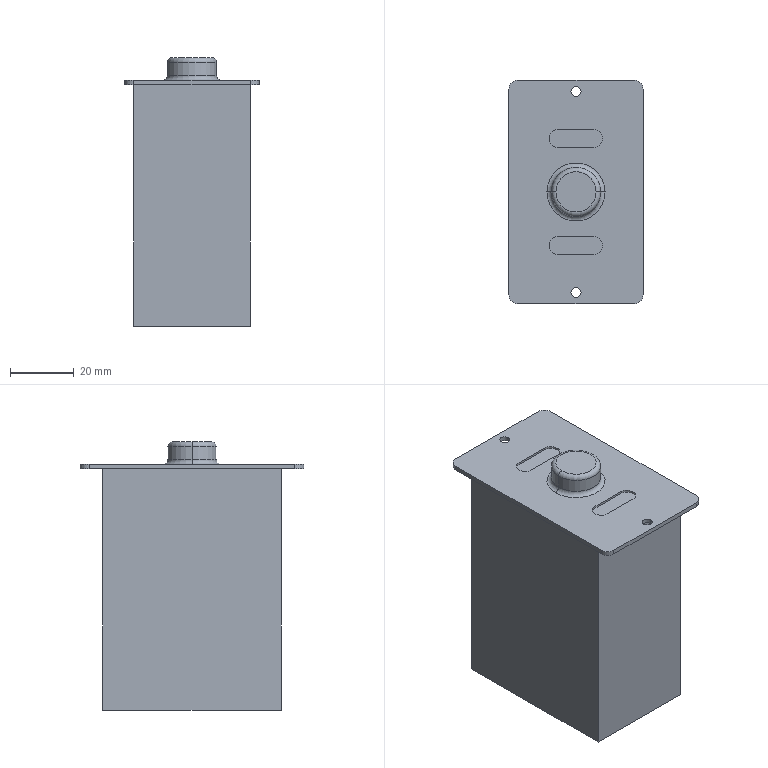Part | SolidWorks | features SplitBody 1 | 1 solid | 38 faces | box 42 x 70 x 84 mm | volume 159371 mm3 | plane 18 | cylinder 16 | torus 4 | commonest cylinder face diameters 5.6 x10 3.15 x4 15.4 x2
STEP:
#1=CARTESIAN_POINT('',(143.875,186.159,-254.516));
#2=VERTEX_POINT('',#1);
#3=CARTESIAN_POINT('',(125.675,186.159,-254.516));
#4=VERTEX_POINT('',#3);
#5=CARTESIAN_POINT('',(134.775,186.159,-254.516));
#6=DIRECTION('',(0.,0.,-1.));
#7=DIRECTION('',(-1.,0.,0.));
#8=AXIS2_PLACEMENT_3D('',#5,#6,#7);
#9=CIRCLE('',#8,9.1);
#10=EDGE_CURVE('',#2,#4,#9,.T.);
#11=ORIENTED_EDGE('',*,*,#10,.F.);
#12=CARTESIAN_POINT('',(142.475,186.159,-253.116));
#13=VERTEX_POINT('',#12);
#14=CARTESIAN_POINT('',(143.875,186.159,-253.116));
#15=DIRECTION('',(0.,1.,0.));
#16=DIRECTION('',(-1.,0.,0.));
#17=AXIS2_PLACEMENT_3D('',#14,#15,#16);
#18=CIRCLE('',#17,1.4);
#19=EDGE_CURVE('',#2,#13,#18,.T.);
#20=ORIENTED_EDGE('',*,*,#19,.T.);
#21=CARTESIAN_POINT('',(127.075,186.159,-253.116));
#22=VERTEX_POINT('',#21);
#23=CARTESIAN_POINT('',(134.775,186.159,-253.116));
#24=DIRECTION('',(0.,0.,1.));
#25=DIRECTION('',(-1.,0.,0.));
#26=AXIS2_PLACEMENT_3D('',#23,#24,#25);
#27=CIRCLE('',#26,7.7);
#28=EDGE_CURVE('',#22,#13,#27,.T.);
#29=ORIENTED_EDGE('',*,*,#28,.F.);
#30=CARTESIAN_POINT('',(125.675,186.159,-253.116));
#31=DIRECTION('',(0.,-1.,0.));
#32=DIRECTION('',(1.,0.,0.));
#33=AXIS2_PLACEMENT_3D('',#30,#31,#32);
#34=CIRCLE('',#33,1.4);
#35=EDGE_CURVE('',#4,#22,#34,.T.);
#36=ORIENTED_EDGE('',*,*,#35,.F.);
#37=EDGE_LOOP('',(#11,#20,#29,#36));
#38=FACE_OUTER_BOUND('',#37,.T.);
#39=CARTESIAN_POINT('',(134.775,186.159,-253.116));
#40=DIRECTION('',(0.,0.,-1.));
#41=DIRECTION('',(-1.,0.,0.));
#42=AXIS2_PLACEMENT_3D('',#39,#40,#41);
#43=TOROIDAL_SURFACE('',#42,9.1,1.4);
#44=ADVANCED_FACE('',(#38),#43,.F.);
#45=CARTESIAN_POINT('',(127.075,186.159,-248.916));
#46=VERTEX_POINT('',#45);
#47=CARTESIAN_POINT('',(142.475,186.159,-248.916));
#48=VERTEX_POINT('',#47);
#49=CARTESIAN_POINT('',(134.775,186.159,-248.916));
#50=DIRECTION('',(0.,0.,-1.));
#51=DIRECTION('',(1.,0.,0.));
#52=AXIS2_PLACEMENT_3D('',#49,#50,#51);
#53=CIRCLE('',#52,7.7);
#54=EDGE_CURVE('',#46,#48,#53,.T.);
#55=ORIENTED_EDGE('',*,*,#54,.F.);
#56=CARTESIAN_POINT('',(128.475,186.159,-247.516));
#57=VERTEX_POINT('',#56);
#58=CARTESIAN_POINT('',(128.475,186.159,-248.916));
#59=DIRECTION('',(0.,1.,0.));
#60=DIRECTION('',(0.,0.,1.));
#61=AXIS2_PLACEMENT_3D('',#58,#59,#60);
#62=CIRCLE('',#61,1.4);
#63=EDGE_CURVE('',#46,#57,#62,.T.);
#64=ORIENTED_EDGE('',*,*,#63,.T.);
#65=CARTESIAN_POINT('',(141.075,186.159,-247.516));
#66=VERTEX_POINT('',#65);
#67=CARTESIAN_POINT('',(134.775,186.159,-247.516));
#68=DIRECTION('',(0.,0.,1.));
#69=DIRECTION('',(1.,0.,0.));
#70=AXIS2_PLACEMENT_3D('',#67,#68,#69);
#71=CIRCLE('',#70,6.3);
#72=EDGE_CURVE('',#66,#57,#71,.T.);
#73=ORIENTED_EDGE('',*,*,#72,.F.);
#74=CARTESIAN_POINT('',(141.075,186.159,-248.916));
#75=DIRECTION('',(0.,-1.,0.));
#76=DIRECTION('',(1.,0.,0.));
#77=AXIS2_PLACEMENT_3D('',#74,#75,#76);
#78=CIRCLE('',#77,1.4);
#79=EDGE_CURVE('',#48,#66,#78,.T.);
#80=ORIENTED_EDGE('',*,*,#79,.F.);
#81=EDGE_LOOP('',(#55,#64,#73,#80));
#82=FACE_OUTER_BOUND('',#81,.T.);
#83=CARTESIAN_POINT('',(134.775,186.159,-248.916));
#84=DIRECTION('',(0.,0.,1.));
#85=DIRECTION('',(1.,0.,0.));
#86=AXIS2_PLACEMENT_3D('',#83,#84,#85);
#87=TOROIDAL_SURFACE('',#86,6.3,1.4);
#88=ADVANCED_FACE('',(#82),#87,.T.);
#89=CARTESIAN_POINT('',(143.175,169.359,-255.216));
#90=VERTEX_POINT('',#89);
#91=CARTESIAN_POINT('',(140.375,172.159,-255.216));
#92=VERTEX_POINT('',#91);
#93=CARTESIAN_POINT('',(140.375,169.359,-255.216));
#94=DIRECTION('',(0.,0.,1.));
#95=DIRECTION('',(-1.,0.,0.));
#96=AXIS2_PLACEMENT_3D('',#93,#94,#95);
#97=CIRCLE('',#96,2.8);
#98=EDGE_CURVE('',#90,#92,#97,.T.);
#99=ORIENTED_EDGE('',*,*,#98,.F.);
#100=CARTESIAN_POINT('',(143.175,169.359,-254.516));
#101=VERTEX_POINT('',#100);
#102=CARTESIAN_POINT('',(143.175,169.359,-255.216));
#103=DIRECTION('',(0.,0.,1.));
#104=VECTOR('',#103,1000.);
#105=LINE('',#102,#104);
#106=EDGE_CURVE('',#90,#101,#105,.T.);
#107=ORIENTED_EDGE('',*,*,#106,.T.);
#108=CARTESIAN_POINT('',(140.375,172.159,-254.516));
#109=VERTEX_POINT('',#108);
#110=CARTESIAN_POINT('',(140.375,169.359,-254.516));
#111=DIRECTION('',(0.,0.,1.));
#112=DIRECTION('',(-1.,0.,0.));
#113=AXIS2_PLACEMENT_3D('',#110,#111,#112);
#114=CIRCLE('',#113,2.8);
#115=EDGE_CURVE('',#101,#109,#114,.T.);
#116=ORIENTED_EDGE('',*,*,#115,.T.);
#117=CARTESIAN_POINT('',(140.375,172.159,-255.216));
#118=DIRECTION('',(0.,0.,1.));
#119=VECTOR('',#118,1000.);
#120=LINE('',#117,#119);
#121=EDGE_CURVE('',#92,#109,#120,.T.);
#122=ORIENTED_EDGE('',*,*,#121,.F.);
#123=EDGE_LOOP('',(#99,#107,#116,#122));
#124=FACE_OUTER_BOUND('',#123,.T.);
#125=CARTESIAN_POINT('',(140.375,169.359,-255.216));
#126=DIRECTION('',(0.,0.,1.));
#127=DIRECTION('',(1.,0.,0.));
#128=AXIS2_PLACEMENT_3D('',#125,#126,#127);
#129=CYLINDRICAL_SURFACE('',#128,2.8);
#130=ADVANCED_FACE('',(#124),#129,.F.);
#131=CARTESIAN_POINT('',(143.175,202.959,-255.216));
#132=VERTEX_POINT('',#131);
#133=CARTESIAN_POINT('',(140.375,205.759,-255.216));
#134=VERTEX_POINT('',#133);
#135=CARTESIAN_POINT('',(140.375,202.959,-255.216));
#136=DIRECTION('',(0.,0.,1.));
#137=DIRECTION('',(1.,0.,0.));
#138=AXIS2_PLACEMENT_3D('',#135,#136,#137);
#139=CIRCLE('',#138,2.8);
#140=EDGE_CURVE('',#132,#134,#139,.T.);
#141=ORIENTED_EDGE('',*,*,#140,.F.);
#142=CARTESIAN_POINT('',(143.175,202.959,-254.516));
#143=VERTEX_POINT('',#142);
#144=CARTESIAN_POINT('',(143.175,202.959,-255.216));
#145=DIRECTION('',(0.,0.,1.));
#146=VECTOR('',#145,1000.);
#147=LINE('',#144,#146);
#148=EDGE_CURVE('',#132,#143,#147,.T.);
#149=ORIENTED_EDGE('',*,*,#148,.T.);
#150=CARTESIAN_POINT('',(140.375,205.759,-254.516));
#151=VERTEX_POINT('',#150);
#152=CARTESIAN_POINT('',(140.375,202.959,-254.516));
#153=DIRECTION('',(0.,0.,1.));
#154=DIRECTION('',(1.,0.,0.));
#155=AXIS2_PLACEMENT_3D('',#152,#153,#154);
#156=CIRCLE('',#155,2.8);
#157=EDGE_CURVE('',#143,#151,#156,.T.);
#158=ORIENTED_EDGE('',*,*,#157,.T.);
#159=CARTESIAN_POINT('',(140.375,205.759,-255.216));
#160=DIRECTION('',(0.,0.,1.));
#161=VECTOR('',#160,1000.);
#162=LINE('',#159,#161);
#163=EDGE_CURVE('',#134,#151,#162,.T.);
#164=ORIENTED_EDGE('',*,*,#163,.F.);
#165=EDGE_LOOP('',(#141,#149,#158,#164));
#166=FACE_OUTER_BOUND('',#165,.T.);
#167=CARTESIAN_POINT('',(140.375,202.959,-255.216));
#168=DIRECTION('',(0.,0.,1.));
#169=DIRECTION('',(1.,0.,0.));
#170=AXIS2_PLACEMENT_3D('',#167,#168,#169);
#171=CYLINDRICAL_SURFACE('',#170,2.8);
#172=ADVANCED_FACE('',(#166),#171,.F.);
#173=ORIENTED_EDGE('',*,*,#54,.T.);
#174=CARTESIAN_POINT('',(142.475,186.159,-247.516));
#175=DIRECTION('',(0.,0.,-1.));
#176=VECTOR('',#175,1000.);
#177=LINE('',#174,#176);
#178=EDGE_CURVE('',#48,#13,#177,.T.);
#179=ORIENTED_EDGE('',*,*,#178,.T.);
#180=CARTESIAN_POINT('',(134.775,186.159,-253.116));
#181=DIRECTION('',(0.,0.,1.));
#182=DIRECTION('',(-1.,0.,0.));
#183=AXIS2_PLACEMENT_3D('',#180,#181,#182);
#184=CIRCLE('',#183,7.7);
#185=EDGE_CURVE('',#13,#22,#184,.T.);
#186=ORIENTED_EDGE('',*,*,#185,.T.);
#187=CARTESIAN_POINT('',(127.075,186.159,-247.516));
#188=DIRECTION('',(0.,0.,-1.));
#189=VECTOR('',#188,1000.);
#190=LINE('',#187,#189);
#191=EDGE_CURVE('',#46,#22,#190,.T.);
#192=ORIENTED_EDGE('',*,*,#191,.F.);
#193=EDGE_LOOP('',(#173,#179,#186,#192));
#194=FACE_OUTER_BOUND('',#193,.T.);
#195=CARTESIAN_POINT('',(134.775,186.159,-247.516));
#196=DIRECTION('',(0.,0.,-1.));
#197=DIRECTION('',(-1.,0.,0.));
#198=AXIS2_PLACEMENT_3D('',#195,#196,#197);
#199=CYLINDRICAL_SURFACE('',#198,7.7);
#200=ADVANCED_FACE('',(#194),#199,.T.);
#201=CARTESIAN_POINT('',(133.2,154.659,-255.916));
#202=VERTEX_POINT('',#201);
#203=CARTESIAN_POINT('',(136.35,154.659,-255.916));
#204=VERTEX_POINT('',#203);
#205=CARTESIAN_POINT('',(134.775,154.659,-255.916));
#206=DIRECTION('',(0.,0.,1.));
#207=DIRECTION('',(1.,0.,0.));
#208=AXIS2_PLACEMENT_3D('',#205,#206,#207);
#209=CIRCLE('',#208,1.575);
#210=EDGE_CURVE('',#202,#204,#209,.T.);
#211=ORIENTED_EDGE('',*,*,#210,.F.);
#212=CARTESIAN_POINT('',(133.2,154.659,-254.516));
#213=VERTEX_POINT('',#212);
#214=CARTESIAN_POINT('',(133.2,154.659,-331.516));
#215=DIRECTION('',(0.,0.,1.));
#216=VECTOR('',#215,1000.);
#217=LINE('',#214,#216);
#218=EDGE_CURVE('',#202,#213,#217,.T.);
#219=ORIENTED_EDGE('',*,*,#218,.T.);
#220=CARTESIAN_POINT('',(136.35,154.659,-254.516));
#221=VERTEX_POINT('',#220);
#222=CARTESIAN_POINT('',(134.775,154.659,-254.516));
#223=DIRECTION('',(0.,0.,1.));
#224=DIRECTION('',(-1.,0.,0.));
#225=AXIS2_PLACEMENT_3D('',#222,#223,#224);
#226=CIRCLE('',#225,1.575);
#227=EDGE_CURVE('',#213,#221,#226,.T.);
#228=ORIENTED_EDGE('',*,*,#227,.T.);
#229=CARTESIAN_POINT('',(136.35,154.659,-331.516));
#230=DIRECTION('',(0.,0.,1.));
#231=VECTOR('',#230,1000.);
#232=LINE('',#229,#231);
#233=EDGE_CURVE('',#204,#221,#232,.T.);
#234=ORIENTED_EDGE('',*,*,#233,.F.);
#235=EDGE_LOOP('',(#211,#219,#228,#234));
#236=FACE_OUTER_BOUND('',#235,.T.);
#237=CARTESIAN_POINT('',(134.775,154.659,-331.516));
#238=DIRECTION('',(0.,0.,1.));
#239=DIRECTION('',(1.,0.,0.));
#240=AXIS2_PLACEMENT_3D('',#237,#238,#239);
#241=CYLINDRICAL_SURFACE('',#240,1.575);
#242=ADVANCED_FACE('',(#236),#241,.F.);
#243=CARTESIAN_POINT('',(133.2,217.659,-255.916));
#244=VERTEX_POINT('',#243);
#245=CARTESIAN_POINT('',(136.35,217.659,-255.916));
#246=VERTEX_POINT('',#245);
#247=CARTESIAN_POINT('',(134.775,217.659,-255.916));
#248=DIRECTION('',(0.,0.,1.));
#249=DIRECTION('',(1.,0.,0.));
#250=AXIS2_PLACEMENT_3D('',#247,#248,#249);
#251=CIRCLE('',#250,1.575);
#252=EDGE_CURVE('',#244,#246,#251,.T.);
#253=ORIENTED_EDGE('',*,*,#252,.F.);
#254=CARTESIAN_POINT('',(133.2,217.659,-254.516));
#255=VERTEX_POINT('',#254);
#256=CARTESIAN_POINT('',(133.2,217.659,-331.516));
#257=DIRECTION('',(0.,0.,1.));
#258=VECTOR('',#257,1000.);
#259=LINE('',#256,#258);
#260=EDGE_CURVE('',#244,#255,#259,.T.);
#261=ORIENTED_EDGE('',*,*,#260,.T.);
#262=CARTESIAN_POINT('',(136.35,217.659,-254.516));
#263=VERTEX_POINT('',#262);
#264=CARTESIAN_POINT('',(134.775,217.659,-254.516));
#265=DIRECTION('',(0.,0.,1.));
#266=DIRECTION('',(1.,0.,0.));
#267=AXIS2_PLACEMENT_3D('',#264,#265,#266);
#268=CIRCLE('',#267,1.575);
#269=EDGE_CURVE('',#255,#263,#268,.T.);
#270=ORIENTED_EDGE('',*,*,#269,.T.);
#271=CARTESIAN_POINT('',(136.35,217.659,-331.516));
#272=DIRECTION('',(0.,0.,1.));
#273=VECTOR('',#272,1000.);
#274=LINE('',#271,#273);
#275=EDGE_CURVE('',#246,#263,#274,.T.);
#276=ORIENTED_EDGE('',*,*,#275,.F.);
#277=EDGE_LOOP('',(#253,#261,#270,#276));
#278=FACE_OUTER_BOUND('',#277,.T.);
#279=CARTESIAN_POINT('',(134.775,217.659,-331.516));
#280=DIRECTION('',(0.,0.,1.));
#281=DIRECTION('',(1.,0.,0.));
#282=AXIS2_PLACEMENT_3D('',#279,#280,#281);
#283=CYLINDRICAL_SURFACE('',#282,1.575);
#284=ADVANCED_FACE('',(#278),#283,.F.);
#285=CARTESIAN_POINT('',(134.775,186.159,-254.516));
#286=DIRECTION('',(0.,0.,-1.));
#287=DIRECTION('',(-1.,0.,0.));
#288=AXIS2_PLACEMENT_3D('',#285,#286,#287);
#289=CIRCLE('',#288,9.1);
#290=EDGE_CURVE('',#4,#2,#289,.T.);
#291=ORIENTED_EDGE('',*,*,#290,.T.);
#292=ORIENTED_EDGE('',*,*,#10,.T.);
#293=EDGE_LOOP('',(#291,#292));
#294=FACE_BOUND('',#293,.T.);
#295=CARTESIAN_POINT('',(129.175,166.559,-254.516));
#296=VERTEX_POINT('',#295);
#297=CARTESIAN_POINT('',(140.375,166.559,-254.516));
#298=VERTEX_POINT('',#297);
#299=CARTESIAN_POINT('',(129.175,166.559,-254.516));
#300=DIRECTION('',(1.,0.,0.));
#301=VECTOR('',#300,1000.);
#302=LINE('',#299,#301);
#303=EDGE_CURVE('',#296,#298,#302,.T.);
#304=ORIENTED_EDGE('',*,*,#303,.F.);
#305=CARTESIAN_POINT('',(129.175,172.159,-254.516));
#306=VERTEX_POINT('',#305);
#307=CARTESIAN_POINT('',(129.175,169.359,-254.516));
#308=DIRECTION('',(0.,0.,1.));
#309=DIRECTION('',(-1.,0.,0.));
#310=AXIS2_PLACEMENT_3D('',#307,#308,#309);
#311=CIRCLE('',#310,2.8);
#312=EDGE_CURVE('',#306,#296,#311,.T.);
#313=ORIENTED_EDGE('',*,*,#312,.F.);
#314=CARTESIAN_POINT('',(129.175,172.159,-254.516));
#315=DIRECTION('',(-1.,0.,0.));
#316=VECTOR('',#315,1000.);
#317=LINE('',#314,#316);
#318=EDGE_CURVE('',#109,#306,#317,.T.);
#319=ORIENTED_EDGE('',*,*,#318,.F.);
#320=ORIENTED_EDGE('',*,*,#115,.F.);
#321=CARTESIAN_POINT('',(140.375,169.359,-254.516));
#322=DIRECTION('',(0.,0.,1.));
#323=DIRECTION('',(-1.,0.,0.));
#324=AXIS2_PLACEMENT_3D('',#321,#322,#323);
#325=CIRCLE('',#324,2.8);
#326=EDGE_CURVE('',#298,#101,#325,.T.);
#327=ORIENTED_EDGE('',*,*,#326,.F.);
#328=EDGE_LOOP('',(#304,#313,#319,#320,#327));
#329=FACE_BOUND('',#328,.T.);
#330=CARTESIAN_POINT('',(129.175,200.159,-254.516));
#331=VERTEX_POINT('',#330);
#332=CARTESIAN_POINT('',(140.375,200.159,-254.516));
#333=VERTEX_POINT('',#332);
#334=CARTESIAN_POINT('',(129.175,200.159,-254.516));
#335=DIRECTION('',(1.,0.,0.));
#336=VECTOR('',#335,1000.);
#337=LINE('',#334,#336);
#338=EDGE_CURVE('',#331,#333,#337,.T.);
#339=ORIENTED_EDGE('',*,*,#338,.F.);
#340=CARTESIAN_POINT('',(129.175,205.759,-254.516));
#341=VERTEX_POINT('',#340);
#342=CARTESIAN_POINT('',(129.175,202.959,-254.516));
#343=DIRECTION('',(0.,0.,1.));
#344=DIRECTION('',(1.,0.,0.));
#345=AXIS2_PLACEMENT_3D('',#342,#343,#344);
#346=CIRCLE('',#345,2.8);
#347=EDGE_CURVE('',#341,#331,#346,.T.);
#348=ORIENTED_EDGE('',*,*,#347,.F.);
#349=CARTESIAN_POINT('',(129.175,205.759,-254.516));
#350=DIRECTION('',(-1.,0.,0.));
#351=VECTOR('',#350,1000.);
#352=LINE('',#349,#351);
#353=EDGE_CURVE('',#151,#341,#352,.T.);
#354=ORIENTED_EDGE('',*,*,#353,.F.);
#355=ORIENTED_EDGE('',*,*,#157,.F.);
#356=CARTESIAN_POINT('',(140.375,202.959,-254.516));
#357=DIRECTION('',(0.,0.,1.));
#358=DIRECTION('',(1.,0.,0.));
#359=AXIS2_PLACEMENT_3D('',#356,#357,#358);
#360=CIRCLE('',#359,2.8);
#361=EDGE_CURVE('',#333,#143,#360,.T.);
#362=ORIENTED_EDGE('',*,*,#361,.F.);
#363=EDGE_LOOP('',(#339,#348,#354,#355,#362));
#364=FACE_BOUND('',#363,.T.);
#365=CARTESIAN_POINT('',(116.575,151.159,-254.516));
#366=VERTEX_POINT('',#365);
#367=CARTESIAN_POINT('',(152.975,151.159,-254.516));
#368=VERTEX_POINT('',#367);
#369=CARTESIAN_POINT('',(113.775,151.159,-254.516));
#370=DIRECTION('',(1.,0.,0.));
#371=VECTOR('',#370,1000.);
#372=LINE('',#369,#371);
#373=EDGE_CURVE('',#366,#368,#372,.T.);
#374=ORIENTED_EDGE('',*,*,#373,.T.);
#375=CARTESIAN_POINT('',(155.775,153.959,-254.516));
#376=VERTEX_POINT('',#375);
#377=CARTESIAN_POINT('',(152.975,153.959,-254.516));
#378=DIRECTION('',(0.,0.,1.));
#379=DIRECTION('',(-1.,0.,0.));
#380=AXIS2_PLACEMENT_3D('',#377,#378,#379);
#381=CIRCLE('',#380,2.8);
#382=EDGE_CURVE('',#368,#376,#381,.T.);
#383=ORIENTED_EDGE('',*,*,#382,.T.);
#384=CARTESIAN_POINT('',(155.775,218.359,-254.516));
#385=VERTEX_POINT('',#384);
#386=CARTESIAN_POINT('',(155.775,221.159,-254.516));
#387=DIRECTION('',(0.,1.,0.));
#388=VECTOR('',#387,1000.);
#389=LINE('',#386,#388);
#390=EDGE_CURVE('',#376,#385,#389,.T.);
#391=ORIENTED_EDGE('',*,*,#390,.T.);
#392=CARTESIAN_POINT('',(152.975,221.159,-254.516));
#393=VERTEX_POINT('',#392);
#394=CARTESIAN_POINT('',(152.975,218.359,-254.516));
#395=DIRECTION('',(0.,0.,1.));
#396=DIRECTION('',(-1.,0.,0.));
#397=AXIS2_PLACEMENT_3D('',#394,#395,#396);
#398=CIRCLE('',#397,2.8);
#399=EDGE_CURVE('',#385,#393,#398,.T.);
#400=ORIENTED_EDGE('',*,*,#399,.T.);
#401=CARTESIAN_POINT('',(116.575,221.159,-254.516));
#402=VERTEX_POINT('',#401);
#403=CARTESIAN_POINT('',(113.775,221.159,-254.516));
#404=DIRECTION('',(-1.,0.,0.));
#405=VECTOR('',#404,1000.);
#406=LINE('',#403,#405);
#407=EDGE_CURVE('',#393,#402,#406,.T.);
#408=ORIENTED_EDGE('',*,*,#407,.T.);
#409=CARTESIAN_POINT('',(113.775,218.359,-254.516));
#410=VERTEX_POINT('',#409);
#411=CARTESIAN_POINT('',(116.575,218.359,-254.516));
#412=DIRECTION('',(0.,0.,1.));
#413=DIRECTION('',(-1.,0.,0.));
#414=AXIS2_PLACEMENT_3D('',#411,#412,#413);
#415=CIRCLE('',#414,2.8);
#416=EDGE_CURVE('',#402,#410,#415,.T.);
#417=ORIENTED_EDGE('',*,*,#416,.T.);
#418=CARTESIAN_POINT('',(113.775,153.959,-254.516));
#419=VERTEX_POINT('',#418);
#420=CARTESIAN_POINT('',(113.775,221.159,-254.516));
#421=DIRECTION('',(0.,-1.,0.));
#422=VECTOR('',#421,1000.);
#423=LINE('',#420,#422);
#424=EDGE_CURVE('',#410,#419,#423,.T.);
#425=ORIENTED_EDGE('',*,*,#424,.T.);
#426=CARTESIAN_POINT('',(116.575,153.959,-254.516));
#427=DIRECTION('',(0.,0.,1.));
#428=DIRECTION('',(-1.,0.,0.));
#429=AXIS2_PLACEMENT_3D('',#426,#427,#428);
#430=CIRCLE('',#429,2.8);
#431=EDGE_CURVE('',#419,#366,#430,.T.);
#432=ORIENTED_EDGE('',*,*,#431,.T.);
#433=EDGE_LOOP('',(#374,#383,#391,#400,#408,#417,#425,#432));
#434=FACE_OUTER_BOUND('',#433,.T.);
#435=CARTESIAN_POINT('',(134.775,217.659,-254.516));
#436=DIRECTION('',(0.,0.,1.));
#437=DIRECTION('',(1.,0.,0.));
#438=AXIS2_PLACEMENT_3D('',#435,#436,#437);
#439=CIRCLE('',#438,1.575);
#440=EDGE_CURVE('',#263,#255,#439,.T.);
#441=ORIENTED_EDGE('',*,*,#440,.F.);
#442=ORIENTED_EDGE('',*,*,#269,.F.);
#443=EDGE_LOOP('',(#441,#442));
#444=FACE_BOUND('',#443,.T.);
#445=CARTESIAN_POINT('',(134.775,154.659,-254.516));
#446=DIRECTION('',(0.,0.,1.));
#447=DIRECTION('',(-1.,0.,0.));
#448=AXIS2_PLACEMENT_3D('',#445,#446,#447);
#449=CIRCLE('',#448,1.575);
#450=EDGE_CURVE('',#221,#213,#449,.T.);
#451=ORIENTED_EDGE('',*,*,#450,.F.);
#452=ORIENTED_EDGE('',*,*,#227,.F.);
#453=EDGE_LOOP('',(#451,#452));
#454=FACE_BOUND('',#453,.T.);
#455=CARTESIAN_POINT('',(152.975,158.159,-254.516));
#456=DIRECTION('',(0.,0.,-1.));
#457=DIRECTION('',(-1.,0.,0.));
#458=AXIS2_PLACEMENT_3D('',#455,#456,#457);
#459=PLANE('',#458);
#460=ADVANCED_FACE('',(#294,#329,#364,#434,#444,#454),#459,.F.);
#461=CARTESIAN_POINT('',(152.975,158.159,-255.916));
#462=VERTEX_POINT('',#461);
#463=CARTESIAN_POINT('',(152.975,214.159,-255.916));
#464=VERTEX_POINT('',#463);
#465=CARTESIAN_POINT('',(152.975,214.159,-255.916));
#466=DIRECTION('',(0.,1.,0.));
#467=VECTOR('',#466,1000.);
#468=LINE('',#465,#467);
#469=EDGE_CURVE('',#462,#464,#468,.T.);
#470=ORIENTED_EDGE('',*,*,#469,.F.);
#471=CARTESIAN_POINT('',(152.975,158.159,-331.516));
#472=VERTEX_POINT('',#471);
#473=CARTESIAN_POINT('',(152.975,158.159,-331.516));
#474=DIRECTION('',(0.,0.,1.));
#475=VECTOR('',#474,1000.);
#476=LINE('',#473,#475);
#477=EDGE_CURVE('',#472,#462,#476,.T.);
#478=ORIENTED_EDGE('',*,*,#477,.F.);
#479=CARTESIAN_POINT('',(152.975,214.159,-331.516));
#480=VERTEX_POINT('',#479);
#481=CARTESIAN_POINT('',(152.975,214.159,-331.516));
#482=DIRECTION('',(0.,-1.,0.));
#483=VECTOR('',#482,1000.);
#484=LINE('',#481,#483);
#485=EDGE_CURVE('',#480,#472,#484,.T.);
#486=ORIENTED_EDGE('',*,*,#485,.F.);
#487=CARTESIAN_POINT('',(152.975,214.159,-331.516));
#488=DIRECTION('',(0.,0.,1.));
#489=VECTOR('',#488,1000.);
#490=LINE('',#487,#489);
#491=EDGE_CURVE('',#480,#464,#490,.T.);
#492=ORIENTED_EDGE('',*,*,#491,.T.);
#493=EDGE_LOOP('',(#470,#478,#486,#492));
#494=FACE_OUTER_BOUND('',#493,.T.);
#495=CARTESIAN_POINT('',(152.975,214.159,-331.516));
#496=DIRECTION('',(-1.,0.,0.));
#497=DIRECTION('',(0.,1.,0.));
#498=AXIS2_PLACEMENT_3D('',#495,#496,#497);
#499=PLANE('',#498);
#500=ADVANCED_FACE('',(#494),#499,.F.);
#501=CARTESIAN_POINT('',(116.575,158.159,-255.916));
#502=VERTEX_POINT('',#501);
#503=CARTESIAN_POINT('',(152.975,158.159,-255.916));
#504=DIRECTION('',(1.,0.,0.));
#505=VECTOR('',#504,1000.);
#506=LINE('',#503,#505);
#507=EDGE_CURVE('',#502,#462,#506,.T.);
#508=ORIENTED_EDGE('',*,*,#507,.F.);
#509=CARTESIAN_POINT('',(116.575,158.159,-331.516));
#510=VERTEX_POINT('',#509);
#511=CARTESIAN_POINT('',(116.575,158.159,-331.516));
#512=DIRECTION('',(0.,0.,1.));
#513=VECTOR('',#512,1000.);
#514=LINE('',#511,#513);
#515=EDGE_CURVE('',#510,#502,#514,.T.);
#516=ORIENTED_EDGE('',*,*,#515,.F.);
#517=CARTESIAN_POINT('',(152.975,158.159,-331.516));
#518=DIRECTION('',(-1.,0.,0.));
#519=VECTOR('',#518,1000.);
#520=LINE('',#517,#519);
#521=EDGE_CURVE('',#472,#510,#520,.T.);
#522=ORIENTED_EDGE('',*,*,#521,.F.);
#523=ORIENTED_EDGE('',*,*,#477,.T.);
#524=EDGE_LOOP('',(#508,#516,#522,#523));
#525=FACE_OUTER_BOUND('',#524,.T.);
#526=CARTESIAN_POINT('',(152.975,158.159,-331.516));
#527=DIRECTION('',(0.,1.,0.));
#528=DIRECTION('',(0.,0.,-1.));
#529=AXIS2_PLACEMENT_3D('',#526,#527,#528);
#530=PLANE('',#529);
#531=ADVANCED_FACE('',(#525),#530,.F.);
#532=CARTESIAN_POINT('',(116.575,214.159,-255.916));
#533=VERTEX_POINT('',#532);
#534=CARTESIAN_POINT('',(116.575,214.159,-255.916));
#535=DIRECTION('',(0.,-1.,0.));
#536=VECTOR('',#535,1000.);
#537=LINE('',#534,#536);
#538=EDGE_CURVE('',#533,#502,#537,.T.);
#539=ORIENTED_EDGE('',*,*,#538,.F.);
#540=CARTESIAN_POINT('',(116.575,214.159,-331.516));
#541=VERTEX_POINT('',#540);
#542=CARTESIAN_POINT('',(116.575,214.159,-331.516));
#543=DIRECTION('',(0.,0.,1.));
#544=VECTOR('',#543,1000.);
#545=LINE('',#542,#544);
#546=EDGE_CURVE('',#541,#533,#545,.T.);
#547=ORIENTED_EDGE('',*,*,#546,.F.);
#548=CARTESIAN_POINT('',(116.575,214.159,-331.516));
#549=DIRECTION('',(0.,1.,0.));
#550=VECTOR('',#549,1000.);
#551=LINE('',#548,#550);
#552=EDGE_CURVE('',#510,#541,#551,.T.);
#553=ORIENTED_EDGE('',*,*,#552,.F.);
#554=ORIENTED_EDGE('',*,*,#515,.T.);
#555=EDGE_LOOP('',(#539,#547,#553,#554));
#556=FACE_OUTER_BOUND('',#555,.T.);
#557=CARTESIAN_POINT('',(116.575,214.159,-331.516));
#558=DIRECTION('',(1.,0.,0.));
#559=DIRECTION('',(0.,-1.,0.));
#560=AXIS2_PLACEMENT_3D('',#557,#558,#559);
#561=PLANE('',#560);
#562=ADVANCED_FACE('',(#556),#561,.F.);
#563=CARTESIAN_POINT('',(152.975,214.159,-255.916));
#564=DIRECTION('',(-1.,0.,0.));
#565=VECTOR('',#564,1000.);
#566=LINE('',#563,#565);
#567=EDGE_CURVE('',#464,#533,#566,.T.);
#568=ORIENTED_EDGE('',*,*,#567,.F.);
#569=ORIENTED_EDGE('',*,*,#491,.F.);
#570=CARTESIAN_POINT('',(152.975,214.159,-331.516));
#571=DIRECTION('',(1.,0.,0.));
#572=VECTOR('',#571,1000.);
#573=LINE('',#570,#572);
#574=EDGE_CURVE('',#541,#480,#573,.T.);
#575=ORIENTED_EDGE('',*,*,#574,.F.);
#576=ORIENTED_EDGE('',*,*,#546,.T.);
#577=EDGE_LOOP('',(#568,#569,#575,#576));
#578=FACE_OUTER_BOUND('',#577,.T.);
#579=CARTESIAN_POINT('',(152.975,214.159,-331.516));
#580=DIRECTION('',(0.,-1.,0.));
#581=DIRECTION('',(0.,0.,1.));
#582=AXIS2_PLACEMENT_3D('',#579,#580,#581);
#583=PLANE('',#582);
#584=ADVANCED_FACE('',(#578),#583,.F.);
#585=ORIENTED_EDGE('',*,*,#485,.T.);
#586=ORIENTED_EDGE('',*,*,#521,.T.);
#587=ORIENTED_EDGE('',*,*,#552,.T.);
#588=ORIENTED_EDGE('',*,*,#574,.T.);
#589=EDGE_LOOP('',(#585,#586,#587,#588));
#590=FACE_OUTER_BOUND('',#589,.T.);
#591=CARTESIAN_POINT('',(152.975,158.159,-331.516));
#592=DIRECTION('',(0.,0.,-1.));
#593=DIRECTION('',(-1.,0.,0.));
#594=AXIS2_PLACEMENT_3D('',#591,#592,#593);
#595=PLANE('',#594);
#596=ADVANCED_FACE('',(#590),#595,.T.);
#597=CARTESIAN_POINT('',(134.775,154.659,-255.916));
#598=DIRECTION('',(0.,0.,1.));
#599=DIRECTION('',(1.,0.,0.));
#600=AXIS2_PLACEMENT_3D('',#597,#598,#599);
#601=CIRCLE('',#600,1.575);
#602=EDGE_CURVE('',#204,#202,#601,.T.);
#603=ORIENTED_EDGE('',*,*,#602,.T.);
#604=ORIENTED_EDGE('',*,*,#210,.T.);
#605=EDGE_LOOP('',(#603,#604));
#606=FACE_BOUND('',#605,.T.);
#607=CARTESIAN_POINT('',(134.775,217.659,-255.916));
#608=DIRECTION('',(0.,0.,1.));
#609=DIRECTION('',(1.,0.,0.));
#610=AXIS2_PLACEMENT_3D('',#607,#608,#609);
#611=CIRCLE('',#610,1.575);
#612=EDGE_CURVE('',#246,#244,#611,.T.);
#613=ORIENTED_EDGE('',*,*,#612,.T.);
#614=ORIENTED_EDGE('',*,*,#252,.T.);
#615=EDGE_LOOP('',(#613,#614));
#616=FACE_BOUND('',#615,.T.);
#617=CARTESIAN_POINT('',(155.775,153.959,-255.916));
#618=VERTEX_POINT('',#617);
#619=CARTESIAN_POINT('',(155.775,218.359,-255.916));
#620=VERTEX_POINT('',#619);
#621=CARTESIAN_POINT('',(155.775,221.159,-255.916));
#622=DIRECTION('',(0.,1.,0.));
#623=VECTOR('',#622,1000.);
#624=LINE('',#621,#623);
#625=EDGE_CURVE('',#618,#620,#624,.T.);
#626=ORIENTED_EDGE('',*,*,#625,.F.);
#627=CARTESIAN_POINT('',(152.975,151.159,-255.916));
#628=VERTEX_POINT('',#627);
#629=CARTESIAN_POINT('',(152.975,153.959,-255.916));
#630=DIRECTION('',(0.,0.,-1.));
#631=DIRECTION('',(1.,0.,0.));
#632=AXIS2_PLACEMENT_3D('',#629,#630,#631);
#633=CIRCLE('',#632,2.8);
#634=EDGE_CURVE('',#618,#628,#633,.T.);
#635=ORIENTED_EDGE('',*,*,#634,.T.);
#636=CARTESIAN_POINT('',(116.575,151.159,-255.916));
#637=VERTEX_POINT('',#636);
#638=CARTESIAN_POINT('',(113.775,151.159,-255.916));
#639=DIRECTION('',(1.,0.,0.));
#640=VECTOR('',#639,1000.);
#641=LINE('',#638,#640);
#642=EDGE_CURVE('',#637,#628,#641,.T.);
#643=ORIENTED_EDGE('',*,*,#642,.F.);
#644=CARTESIAN_POINT('',(113.775,153.959,-255.916));
#645=VERTEX_POINT('',#644);
#646=CARTESIAN_POINT('',(116.575,153.959,-255.916));
#647=DIRECTION('',(0.,0.,-1.));
#648=DIRECTION('',(1.,0.,0.));
#649=AXIS2_PLACEMENT_3D('',#646,#647,#648);
#650=CIRCLE('',#649,2.8);
#651=EDGE_CURVE('',#637,#645,#650,.T.);
#652=ORIENTED_EDGE('',*,*,#651,.T.);
#653=CARTESIAN_POINT('',(113.775,218.359,-255.916));
#654=VERTEX_POINT('',#653);
#655=CARTESIAN_POINT('',(113.775,221.159,-255.916));
#656=DIRECTION('',(0.,-1.,0.));
#657=VECTOR('',#656,1000.);
#658=LINE('',#655,#657);
#659=EDGE_CURVE('',#654,#645,#658,.T.);
#660=ORIENTED_EDGE('',*,*,#659,.F.);
#661=CARTESIAN_POINT('',(116.575,221.159,-255.916));
#662=VERTEX_POINT('',#661);
#663=CARTESIAN_POINT('',(116.575,218.359,-255.916));
#664=DIRECTION('',(0.,0.,-1.));
#665=DIRECTION('',(1.,0.,0.));
#666=AXIS2_PLACEMENT_3D('',#663,#664,#665);
#667=CIRCLE('',#666,2.8);
#668=EDGE_CURVE('',#654,#662,#667,.T.);
#669=ORIENTED_EDGE('',*,*,#668,.T.);
#670=CARTESIAN_POINT('',(152.975,221.159,-255.916));
#671=VERTEX_POINT('',#670);
#672=CARTESIAN_POINT('',(113.775,221.159,-255.916));
#673=DIRECTION('',(-1.,0.,0.));
#674=VECTOR('',#673,1000.);
#675=LINE('',#672,#674);
#676=EDGE_CURVE('',#671,#662,#675,.T.);
#677=ORIENTED_EDGE('',*,*,#676,.F.);
#678=CARTESIAN_POINT('',(152.975,218.359,-255.916));
#679=DIRECTION('',(0.,0.,-1.));
#680=DIRECTION('',(1.,0.,0.));
#681=AXIS2_PLACEMENT_3D('',#678,#679,#680);
#682=CIRCLE('',#681,2.8);
#683=EDGE_CURVE('',#671,#620,#682,.T.);
#684=ORIENTED_EDGE('',*,*,#683,.T.);
#685=EDGE_LOOP('',(#626,#635,#643,#652,#660,#669,#677,#684));
#686=FACE_OUTER_BOUND('',#685,.T.);
#687=ORIENTED_EDGE('',*,*,#507,.T.);
#688=ORIENTED_EDGE('',*,*,#469,.T.);
#689=ORIENTED_EDGE('',*,*,#567,.T.);
#690=ORIENTED_EDGE('',*,*,#538,.T.);
#691=EDGE_LOOP('',(#687,#688,#689,#690));
#692=FACE_BOUND('',#691,.T.);
#693=CARTESIAN_POINT('',(113.775,151.159,-255.916));
#694=DIRECTION('',(0.,0.,1.));
#695=DIRECTION('',(1.,0.,0.));
#696=AXIS2_PLACEMENT_3D('',#693,#694,#695);
#697=PLANE('',#696);
#698=ADVANCED_FACE('',(#606,#616,#686,#692),#697,.F.);
#699=ORIENTED_EDGE('',*,*,#659,.T.);
#700=CARTESIAN_POINT('',(113.775,153.959,-255.916));
#701=DIRECTION('',(0.,0.,1.));
#702=VECTOR('',#701,1000.);
#703=LINE('',#700,#702);
#704=EDGE_CURVE('',#645,#419,#703,.T.);
#705=ORIENTED_EDGE('',*,*,#704,.T.);
#706=ORIENTED_EDGE('',*,*,#424,.F.);
#707=CARTESIAN_POINT('',(113.775,218.359,-255.916));
#708=DIRECTION('',(0.,0.,-1.));
#709=VECTOR('',#708,1000.);
#710=LINE('',#707,#709);
#711=EDGE_CURVE('',#410,#654,#710,.T.);
#712=ORIENTED_EDGE('',*,*,#711,.T.);
#713=EDGE_LOOP('',(#699,#705,#706,#712));
#714=FACE_OUTER_BOUND('',#713,.T.);
#715=CARTESIAN_POINT('',(113.775,221.159,-255.916));
#716=DIRECTION('',(-1.,0.,0.));
#717=DIRECTION('',(0.,1.,0.));
#718=AXIS2_PLACEMENT_3D('',#715,#716,#717);
#719=PLANE('',#718);
#720=ADVANCED_FACE('',(#714),#719,.T.);
#721=ORIENTED_EDGE('',*,*,#407,.F.);
#722=CARTESIAN_POINT('',(152.975,221.159,-255.916));
#723=DIRECTION('',(0.,0.,-1.));
#724=VECTOR('',#723,1000.);
#725=LINE('',#722,#724);
#726=EDGE_CURVE('',#393,#671,#725,.T.);
#727=ORIENTED_EDGE('',*,*,#726,.T.);
#728=ORIENTED_EDGE('',*,*,#676,.T.);
#729=CARTESIAN_POINT('',(116.575,221.159,-255.916));
#730=DIRECTION('',(0.,0.,1.));
#731=VECTOR('',#730,1000.);
#732=LINE('',#729,#731);
#733=EDGE_CURVE('',#662,#402,#732,.T.);
#734=ORIENTED_EDGE('',*,*,#733,.T.);
#735=EDGE_LOOP('',(#721,#727,#728,#734));
#736=FACE_OUTER_BOUND('',#735,.T.);
#737=CARTESIAN_POINT('',(113.775,221.159,-255.916));
#738=DIRECTION('',(0.,1.,0.));
#739=DIRECTION('',(1.,0.,0.));
#740=AXIS2_PLACEMENT_3D('',#737,#738,#739);
#741=PLANE('',#740);
#742=ADVANCED_FACE('',(#736),#741,.T.);
#743=ORIENTED_EDGE('',*,*,#390,.F.);
#744=CARTESIAN_POINT('',(155.775,153.959,-255.916));
#745=DIRECTION('',(0.,0.,-1.));
#746=VECTOR('',#745,1000.);
#747=LINE('',#744,#746);
#748=EDGE_CURVE('',#376,#618,#747,.T.);
#749=ORIENTED_EDGE('',*,*,#748,.T.);
#750=ORIENTED_EDGE('',*,*,#625,.T.);
#751=CARTESIAN_POINT('',(155.775,218.359,-255.916));
#752=DIRECTION('',(0.,0.,1.));
#753=VECTOR('',#752,1000.);
#754=LINE('',#751,#753);
#755=EDGE_CURVE('',#620,#385,#754,.T.);
#756=ORIENTED_EDGE('',*,*,#755,.T.);
#757=EDGE_LOOP('',(#743,#749,#750,#756));
#758=FACE_OUTER_BOUND('',#757,.T.);
#759=CARTESIAN_POINT('',(155.775,221.159,-255.916));
#760=DIRECTION('',(1.,0.,0.));
#761=DIRECTION('',(0.,0.,-1.));
#762=AXIS2_PLACEMENT_3D('',#759,#760,#761);
#763=PLANE('',#762);
#764=ADVANCED_FACE('',(#758),#763,.T.);
#765=ORIENTED_EDGE('',*,*,#642,.T.);
#766=CARTESIAN_POINT('',(152.975,151.159,-255.916));
#767=DIRECTION('',(0.,0.,1.));
#768=VECTOR('',#767,1000.);
#769=LINE('',#766,#768);
#770=EDGE_CURVE('',#628,#368,#769,.T.);
#771=ORIENTED_EDGE('',*,*,#770,.T.);
#772=ORIENTED_EDGE('',*,*,#373,.F.);
#773=CARTESIAN_POINT('',(116.575,151.159,-255.916));
#774=DIRECTION('',(0.,0.,-1.));
#775=VECTOR('',#774,1000.);
#776=LINE('',#773,#775);
#777=EDGE_CURVE('',#366,#637,#776,.T.);
#778=ORIENTED_EDGE('',*,*,#777,.T.);
#779=EDGE_LOOP('',(#765,#771,#772,#778));
#780=FACE_OUTER_BOUND('',#779,.T.);
#781=CARTESIAN_POINT('',(113.775,151.159,-255.916));
#782=DIRECTION('',(0.,-1.,0.));
#783=DIRECTION('',(0.,0.,1.));
#784=AXIS2_PLACEMENT_3D('',#781,#782,#783);
#785=PLANE('',#784);
#786=ADVANCED_FACE('',(#780),#785,.T.);
#787=ORIENTED_EDGE('',*,*,#260,.F.);
#788=ORIENTED_EDGE('',*,*,#612,.F.);
#789=ORIENTED_EDGE('',*,*,#275,.T.);
#790=ORIENTED_EDGE('',*,*,#440,.T.);
#791=EDGE_LOOP('',(#787,#788,#789,#790));
#792=FACE_OUTER_BOUND('',#791,.T.);
#793=CARTESIAN_POINT('',(134.775,217.659,-331.516));
#794=DIRECTION('',(0.,0.,1.));
#795=DIRECTION('',(1.,0.,0.));
#796=AXIS2_PLACEMENT_3D('',#793,#794,#795);
#797=CYLINDRICAL_SURFACE('',#796,1.575);
#798=ADVANCED_FACE('',(#792),#797,.F.);
#799=ORIENTED_EDGE('',*,*,#218,.F.);
#800=ORIENTED_EDGE('',*,*,#602,.F.);
#801=ORIENTED_EDGE('',*,*,#233,.T.);
#802=ORIENTED_EDGE('',*,*,#450,.T.);
#803=EDGE_LOOP('',(#799,#800,#801,#802));
#804=FACE_OUTER_BOUND('',#803,.T.);
#805=CARTESIAN_POINT('',(134.775,154.659,-331.516));
#806=DIRECTION('',(0.,0.,1.));
#807=DIRECTION('',(1.,0.,0.));
#808=AXIS2_PLACEMENT_3D('',#805,#806,#807);
#809=CYLINDRICAL_SURFACE('',#808,1.575);
#810=ADVANCED_FACE('',(#804),#809,.F.);
#811=ORIENTED_EDGE('',*,*,#634,.F.);
#812=ORIENTED_EDGE('',*,*,#748,.F.);
#813=ORIENTED_EDGE('',*,*,#382,.F.);
#814=ORIENTED_EDGE('',*,*,#770,.F.);
#815=EDGE_LOOP('',(#811,#812,#813,#814));
#816=FACE_OUTER_BOUND('',#815,.T.);
#817=CARTESIAN_POINT('',(152.975,153.959,-255.916));
#818=DIRECTION('',(0.,0.,1.));
#819=DIRECTION('',(1.,0.,0.));
#820=AXIS2_PLACEMENT_3D('',#817,#818,#819);
#821=CYLINDRICAL_SURFACE('',#820,2.8);
#822=ADVANCED_FACE('',(#816),#821,.T.);
#823=ORIENTED_EDGE('',*,*,#651,.F.);
#824=ORIENTED_EDGE('',*,*,#777,.F.);
#825=ORIENTED_EDGE('',*,*,#431,.F.);
#826=ORIENTED_EDGE('',*,*,#704,.F.);
#827=EDGE_LOOP('',(#823,#824,#825,#826));
#828=FACE_OUTER_BOUND('',#827,.T.);
#829=CARTESIAN_POINT('',(116.575,153.959,-255.916));
#830=DIRECTION('',(0.,0.,1.));
#831=DIRECTION('',(1.,0.,0.));
#832=AXIS2_PLACEMENT_3D('',#829,#830,#831);
#833=CYLINDRICAL_SURFACE('',#832,2.8);
#834=ADVANCED_FACE('',(#828),#833,.T.);
#835=ORIENTED_EDGE('',*,*,#683,.F.);
#836=ORIENTED_EDGE('',*,*,#726,.F.);
#837=ORIENTED_EDGE('',*,*,#399,.F.);
#838=ORIENTED_EDGE('',*,*,#755,.F.);
#839=EDGE_LOOP('',(#835,#836,#837,#838));
#840=FACE_OUTER_BOUND('',#839,.T.);
#841=CARTESIAN_POINT('',(152.975,218.359,-255.916));
#842=DIRECTION('',(0.,0.,1.));
#843=DIRECTION('',(1.,0.,0.));
#844=AXIS2_PLACEMENT_3D('',#841,#842,#843);
#845=CYLINDRICAL_SURFACE('',#844,2.8);
#846=ADVANCED_FACE('',(#840),#845,.T.);
#847=ORIENTED_EDGE('',*,*,#668,.F.);
#848=ORIENTED_EDGE('',*,*,#711,.F.);
#849=ORIENTED_EDGE('',*,*,#416,.F.);
#850=ORIENTED_EDGE('',*,*,#733,.F.);
#851=EDGE_LOOP('',(#847,#848,#849,#850));
#852=FACE_OUTER_BOUND('',#851,.T.);
#853=CARTESIAN_POINT('',(116.575,218.359,-255.916));
#854=DIRECTION('',(0.,0.,1.));
#855=DIRECTION('',(1.,0.,0.));
#856=AXIS2_PLACEMENT_3D('',#853,#854,#855);
#857=CYLINDRICAL_SURFACE('',#856,2.8);
#858=ADVANCED_FACE('',(#852),#857,.T.);
#859=ORIENTED_EDGE('',*,*,#178,.F.);
#860=CARTESIAN_POINT('',(134.775,186.159,-248.916));
#861=DIRECTION('',(0.,0.,-1.));
#862=DIRECTION('',(1.,0.,0.));
#863=AXIS2_PLACEMENT_3D('',#860,#861,#862);
#864=CIRCLE('',#863,7.7);
#865=EDGE_CURVE('',#48,#46,#864,.T.);
#866=ORIENTED_EDGE('',*,*,#865,.T.);
#867=ORIENTED_EDGE('',*,*,#191,.T.);
#868=ORIENTED_EDGE('',*,*,#28,.T.);
#869=EDGE_LOOP('',(#859,#866,#867,#868));
#870=FACE_OUTER_BOUND('',#869,.T.);
#871=CARTESIAN_POINT('',(134.775,186.159,-247.516));
#872=DIRECTION('',(0.,0.,-1.));
#873=DIRECTION('',(-1.,0.,0.));
#874=AXIS2_PLACEMENT_3D('',#871,#872,#873);
#875=CYLINDRICAL_SURFACE('',#874,7.7);
#876=ADVANCED_FACE('',(#870),#875,.T.);
#877=ORIENTED_EDGE('',*,*,#72,.T.);
#878=CARTESIAN_POINT('',(134.775,186.159,-247.516));
#879=DIRECTION('',(0.,0.,1.));
#880=DIRECTION('',(1.,0.,0.));
#881=AXIS2_PLACEMENT_3D('',#878,#879,#880);
#882=CIRCLE('',#881,6.3);
#883=EDGE_CURVE('',#57,#66,#882,.T.);
#884=ORIENTED_EDGE('',*,*,#883,.T.);
#885=EDGE_LOOP('',(#877,#884));
#886=FACE_OUTER_BOUND('',#885,.T.);
#887=CARTESIAN_POINT('',(134.775,186.159,-247.516));
#888=DIRECTION('',(0.,0.,1.));
#889=DIRECTION('',(1.,0.,0.));
#890=AXIS2_PLACEMENT_3D('',#887,#888,#889);
#891=PLANE('',#890);
#892=ADVANCED_FACE('',(#886),#891,.T.);
#893=ORIENTED_EDGE('',*,*,#347,.T.);
#894=CARTESIAN_POINT('',(129.175,200.159,-255.216));
#895=VERTEX_POINT('',#894);
#896=CARTESIAN_POINT('',(129.175,200.159,-255.216));
#897=DIRECTION('',(0.,0.,1.));
#898=VECTOR('',#897,1000.);
#899=LINE('',#896,#898);
#900=EDGE_CURVE('',#895,#331,#899,.T.);
#901=ORIENTED_EDGE('',*,*,#900,.F.);
#902=CARTESIAN_POINT('',(129.175,205.759,-255.216));
#903=VERTEX_POINT('',#902);
#904=CARTESIAN_POINT('',(129.175,202.959,-255.216));
#905=DIRECTION('',(0.,0.,1.));
#906=DIRECTION('',(1.,0.,0.));
#907=AXIS2_PLACEMENT_3D('',#904,#905,#906);
#908=CIRCLE('',#907,2.8);
#909=EDGE_CURVE('',#903,#895,#908,.T.);
#910=ORIENTED_EDGE('',*,*,#909,.F.);
#911=CARTESIAN_POINT('',(129.175,205.759,-255.216));
#912=DIRECTION('',(0.,0.,1.));
#913=VECTOR('',#912,1000.);
#914=LINE('',#911,#913);
#915=EDGE_CURVE('',#903,#341,#914,.T.);
#916=ORIENTED_EDGE('',*,*,#915,.T.);
#917=EDGE_LOOP('',(#893,#901,#910,#916));
#918=FACE_OUTER_BOUND('',#917,.T.);
#919=CARTESIAN_POINT('',(129.175,202.959,-255.216));
#920=DIRECTION('',(0.,0.,1.));
#921=DIRECTION('',(1.,0.,0.));
#922=AXIS2_PLACEMENT_3D('',#919,#920,#921);
#923=CYLINDRICAL_SURFACE('',#922,2.8);
#924=ADVANCED_FACE('',(#918),#923,.F.);
#925=ORIENTED_EDGE('',*,*,#353,.T.);
#926=ORIENTED_EDGE('',*,*,#915,.F.);
#927=CARTESIAN_POINT('',(129.175,205.759,-255.216));
#928=DIRECTION('',(-1.,0.,0.));
#929=VECTOR('',#928,1000.);
#930=LINE('',#927,#929);
#931=EDGE_CURVE('',#134,#903,#930,.T.);
#932=ORIENTED_EDGE('',*,*,#931,.F.);
#933=ORIENTED_EDGE('',*,*,#163,.T.);
#934=EDGE_LOOP('',(#925,#926,#932,#933));
#935=FACE_OUTER_BOUND('',#934,.T.);
#936=CARTESIAN_POINT('',(129.175,205.759,-255.216));
#937=DIRECTION('',(0.,1.,0.));
#938=DIRECTION('',(1.,0.,0.));
#939=AXIS2_PLACEMENT_3D('',#936,#937,#938);
#940=PLANE('',#939);
#941=ADVANCED_FACE('',(#935),#940,.F.);
#942=ORIENTED_EDGE('',*,*,#148,.F.);
#943=CARTESIAN_POINT('',(140.375,200.159,-255.216));
#944=VERTEX_POINT('',#943);
#945=CARTESIAN_POINT('',(140.375,202.959,-255.216));
#946=DIRECTION('',(0.,0.,1.));
#947=DIRECTION('',(1.,0.,0.));
#948=AXIS2_PLACEMENT_3D('',#945,#946,#947);
#949=CIRCLE('',#948,2.8);
#950=EDGE_CURVE('',#944,#132,#949,.T.);
#951=ORIENTED_EDGE('',*,*,#950,.F.);
#952=CARTESIAN_POINT('',(140.375,200.159,-255.216));
#953=DIRECTION('',(0.,0.,1.));
#954=VECTOR('',#953,1000.);
#955=LINE('',#952,#954);
#956=EDGE_CURVE('',#944,#333,#955,.T.);
#957=ORIENTED_EDGE('',*,*,#956,.T.);
#958=ORIENTED_EDGE('',*,*,#361,.T.);
#959=EDGE_LOOP('',(#942,#951,#957,#958));
#960=FACE_OUTER_BOUND('',#959,.T.);
#961=CARTESIAN_POINT('',(140.375,202.959,-255.216));
#962=DIRECTION('',(0.,0.,1.));
#963=DIRECTION('',(1.,0.,0.));
#964=AXIS2_PLACEMENT_3D('',#961,#962,#963);
#965=CYLINDRICAL_SURFACE('',#964,2.8);
#966=ADVANCED_FACE('',(#960),#965,.F.);
#967=ORIENTED_EDGE('',*,*,#338,.T.);
#968=ORIENTED_EDGE('',*,*,#956,.F.);
#969=CARTESIAN_POINT('',(129.175,200.159,-255.216));
#970=DIRECTION('',(1.,0.,0.));
#971=VECTOR('',#970,1000.);
#972=LINE('',#969,#971);
#973=EDGE_CURVE('',#895,#944,#972,.T.);
#974=ORIENTED_EDGE('',*,*,#973,.F.);
#975=ORIENTED_EDGE('',*,*,#900,.T.);
#976=EDGE_LOOP('',(#967,#968,#974,#975));
#977=FACE_OUTER_BOUND('',#976,.T.);
#978=CARTESIAN_POINT('',(129.175,200.159,-255.216));
#979=DIRECTION('',(0.,-1.,0.));
#980=DIRECTION('',(0.,0.,1.));
#981=AXIS2_PLACEMENT_3D('',#978,#979,#980);
#982=PLANE('',#981);
#983=ADVANCED_FACE('',(#977),#982,.F.);
#984=ORIENTED_EDGE('',*,*,#909,.T.);
#985=ORIENTED_EDGE('',*,*,#973,.T.);
#986=ORIENTED_EDGE('',*,*,#950,.T.);
#987=ORIENTED_EDGE('',*,*,#140,.T.);
#988=ORIENTED_EDGE('',*,*,#931,.T.);
#989=EDGE_LOOP('',(#984,#985,#986,#987,#988));
#990=FACE_OUTER_BOUND('',#989,.T.);
#991=CARTESIAN_POINT('',(129.175,202.959,-255.216));
#992=DIRECTION('',(0.,0.,1.));
#993=DIRECTION('',(1.,0.,0.));
#994=AXIS2_PLACEMENT_3D('',#991,#992,#993);
#995=PLANE('',#994);
#996=ADVANCED_FACE('',(#990),#995,.T.);
#997=ORIENTED_EDGE('',*,*,#312,.T.);
#998=CARTESIAN_POINT('',(129.175,166.559,-255.216));
#999=VERTEX_POINT('',#998);
#1000=CARTESIAN_POINT('',(129.175,166.559,-255.216));
#1001=DIRECTION('',(0.,0.,1.));
#1002=VECTOR('',#1001,1000.);
#1003=LINE('',#1000,#1002);
#1004=EDGE_CURVE('',#999,#296,#1003,.T.);
#1005=ORIENTED_EDGE('',*,*,#1004,.F.);
#1006=CARTESIAN_POINT('',(129.175,172.159,-255.216));
#1007=VERTEX_POINT('',#1006);
#1008=CARTESIAN_POINT('',(129.175,169.359,-255.216));
#1009=DIRECTION('',(0.,0.,1.));
#1010=DIRECTION('',(-1.,0.,0.));
#1011=AXIS2_PLACEMENT_3D('',#1008,#1009,#1010);
#1012=CIRCLE('',#1011,2.8);
#1013=EDGE_CURVE('',#1007,#999,#1012,.T.);
#1014=ORIENTED_EDGE('',*,*,#1013,.F.);
#1015=CARTESIAN_POINT('',(129.175,172.159,-255.216));
#1016=DIRECTION('',(0.,0.,1.));
#1017=VECTOR('',#1016,1000.);
#1018=LINE('',#1015,#1017);
#1019=EDGE_CURVE('',#1007,#306,#1018,.T.);
#1020=ORIENTED_EDGE('',*,*,#1019,.T.);
#1021=EDGE_LOOP('',(#997,#1005,#1014,#1020));
#1022=FACE_OUTER_BOUND('',#1021,.T.);
#1023=CARTESIAN_POINT('',(129.175,169.359,-255.216));
#1024=DIRECTION('',(0.,0.,1.));
#1025=DIRECTION('',(1.,0.,0.));
#1026=AXIS2_PLACEMENT_3D('',#1023,#1024,#1025);
#1027=CYLINDRICAL_SURFACE('',#1026,2.8);
#1028=ADVANCED_FACE('',(#1022),#1027,.F.);
#1029=ORIENTED_EDGE('',*,*,#318,.T.);
#1030=ORIENTED_EDGE('',*,*,#1019,.F.);
#1031=CARTESIAN_POINT('',(129.175,172.159,-255.216));
#1032=DIRECTION('',(-1.,0.,0.));
#1033=VECTOR('',#1032,1000.);
#1034=LINE('',#1031,#1033);
#1035=EDGE_CURVE('',#92,#1007,#1034,.T.);
#1036=ORIENTED_EDGE('',*,*,#1035,.F.);
#1037=ORIENTED_EDGE('',*,*,#121,.T.);
#1038=EDGE_LOOP('',(#1029,#1030,#1036,#1037));
#1039=FACE_OUTER_BOUND('',#1038,.T.);
#1040=CARTESIAN_POINT('',(129.175,172.159,-255.216));
#1041=DIRECTION('',(0.,1.,0.));
#1042=DIRECTION('',(0.,0.,-1.));
#1043=AXIS2_PLACEMENT_3D('',#1040,#1041,#1042);
#1044=PLANE('',#1043);
#1045=ADVANCED_FACE('',(#1039),#1044,.F.);
#1046=ORIENTED_EDGE('',*,*,#106,.F.);
#1047=CARTESIAN_POINT('',(140.375,166.559,-255.216));
#1048=VERTEX_POINT('',#1047);
#1049=CARTESIAN_POINT('',(140.375,169.359,-255.216));
#1050=DIRECTION('',(0.,0.,1.));
#1051=DIRECTION('',(-1.,0.,0.));
#1052=AXIS2_PLACEMENT_3D('',#1049,#1050,#1051);
#1053=CIRCLE('',#1052,2.8);
#1054=EDGE_CURVE('',#1048,#90,#1053,.T.);
#1055=ORIENTED_EDGE('',*,*,#1054,.F.);
#1056=CARTESIAN_POINT('',(140.375,166.559,-255.216));
#1057=DIRECTION('',(0.,0.,1.));
#1058=VECTOR('',#1057,1000.);
#1059=LINE('',#1056,#1058);
#1060=EDGE_CURVE('',#1048,#298,#1059,.T.);
#1061=ORIENTED_EDGE('',*,*,#1060,.T.);
#1062=ORIENTED_EDGE('',*,*,#326,.T.);
#1063=EDGE_LOOP('',(#1046,#1055,#1061,#1062));
#1064=FACE_OUTER_BOUND('',#1063,.T.);
#1065=CARTESIAN_POINT('',(140.375,169.359,-255.216));
#1066=DIRECTION('',(0.,0.,1.));
#1067=DIRECTION('',(1.,0.,0.));
#1068=AXIS2_PLACEMENT_3D('',#1065,#1066,#1067);
#1069=CYLINDRICAL_SURFACE('',#1068,2.8);
#1070=ADVANCED_FACE('',(#1064),#1069,.F.);
#1071=ORIENTED_EDGE('',*,*,#303,.T.);
#1072=ORIENTED_EDGE('',*,*,#1060,.F.);
#1073=CARTESIAN_POINT('',(129.175,166.559,-255.216));
#1074=DIRECTION('',(1.,0.,0.));
#1075=VECTOR('',#1074,1000.);
#1076=LINE('',#1073,#1075);
#1077=EDGE_CURVE('',#999,#1048,#1076,.T.);
#1078=ORIENTED_EDGE('',*,*,#1077,.F.);
#1079=ORIENTED_EDGE('',*,*,#1004,.T.);
#1080=EDGE_LOOP('',(#1071,#1072,#1078,#1079));
#1081=FACE_OUTER_BOUND('',#1080,.T.);
#1082=CARTESIAN_POINT('',(129.175,166.559,-255.216));
#1083=DIRECTION('',(0.,-1.,0.));
#1084=DIRECTION('',(0.,0.,1.));
#1085=AXIS2_PLACEMENT_3D('',#1082,#1083,#1084);
#1086=PLANE('',#1085);
#1087=ADVANCED_FACE('',(#1081),#1086,.F.);
#1088=ORIENTED_EDGE('',*,*,#1013,.T.);
#1089=ORIENTED_EDGE('',*,*,#1077,.T.);
#1090=ORIENTED_EDGE('',*,*,#1054,.T.);
#1091=ORIENTED_EDGE('',*,*,#98,.T.);
#1092=ORIENTED_EDGE('',*,*,#1035,.T.);
#1093=EDGE_LOOP('',(#1088,#1089,#1090,#1091,#1092));
#1094=FACE_OUTER_BOUND('',#1093,.T.);
#1095=CARTESIAN_POINT('',(129.175,169.359,-255.216));
#1096=DIRECTION('',(0.,0.,-1.));
#1097=DIRECTION('',(-1.,0.,0.));
#1098=AXIS2_PLACEMENT_3D('',#1095,#1096,#1097);
#1099=PLANE('',#1098);
#1100=ADVANCED_FACE('',(#1094),#1099,.F.);
#1101=ORIENTED_EDGE('',*,*,#63,.F.);
#1102=ORIENTED_EDGE('',*,*,#865,.F.);
#1103=ORIENTED_EDGE('',*,*,#79,.T.);
#1104=ORIENTED_EDGE('',*,*,#883,.F.);
#1105=EDGE_LOOP('',(#1101,#1102,#1103,#1104));
#1106=FACE_OUTER_BOUND('',#1105,.T.);
#1107=CARTESIAN_POINT('',(134.775,186.159,-248.916));
#1108=DIRECTION('',(0.,0.,1.));
#1109=DIRECTION('',(1.,0.,0.));
#1110=AXIS2_PLACEMENT_3D('',#1107,#1108,#1109);
#1111=TOROIDAL_SURFACE('',#1110,6.3,1.4);
#1112=ADVANCED_FACE('',(#1106),#1111,.T.);
#1113=ORIENTED_EDGE('',*,*,#19,.F.);
#1114=ORIENTED_EDGE('',*,*,#290,.F.);
#1115=ORIENTED_EDGE('',*,*,#35,.T.);
#1116=ORIENTED_EDGE('',*,*,#185,.F.);
#1117=EDGE_LOOP('',(#1113,#1114,#1115,#1116));
#1118=FACE_OUTER_BOUND('',#1117,.T.);
#1119=CARTESIAN_POINT('',(134.775,186.159,-253.116));
#1120=DIRECTION('',(0.,0.,-1.));
#1121=DIRECTION('',(-1.,0.,0.));
#1122=AXIS2_PLACEMENT_3D('',#1119,#1120,#1121);
#1123=TOROIDAL_SURFACE('',#1122,9.1,1.4);
#1124=ADVANCED_FACE('',(#1118),#1123,.F.);
#1125=CLOSED_SHELL('',(#44,#88,#130,#172,#200,#242,#284,#460,#500,#531,#562,#584,#596,#698,#720,#742,#764,#786,#798,#810,#822,#834,#846,#858,#876,#892,#924,#941,#966,#983,#996,#1028,#1045,#1070,#1087,#1100,#1112,#1124));
#1126=MANIFOLD_SOLID_BREP('',#1125);
#1127=CARTESIAN_POINT('',(0.,0.,0.));
#1128=DIRECTION('',(0.,0.,1.));
#1129=DIRECTION('',(1.,0.,0.));
#1130=AXIS2_PLACEMENT_3D('',#1127,#1128,#1129);
#1131=(LENGTH_UNIT()NAMED_UNIT(*)SI_UNIT(.MILLI.,.METRE.));
#1132=UNCERTAINTY_MEASURE_WITH_UNIT(LENGTH_MEASURE(0.00001),#1131,'','');
#1133=(NAMED_UNIT(*)PLANE_ANGLE_UNIT()SI_UNIT($,.RADIAN.));
#1134=(NAMED_UNIT(*)SI_UNIT($,.STERADIAN.)SOLID_ANGLE_UNIT());
#1135=(GEOMETRIC_REPRESENTATION_CONTEXT(3)GLOBAL_UNCERTAINTY_ASSIGNED_CONTEXT((#1132))GLOBAL_UNIT_ASSIGNED_CONTEXT((#1131,#1133,#1134))REPRESENTATION_CONTEXT('',''));
#1136=ADVANCED_BREP_SHAPE_REPRESENTATION('',(#1126,#1130),#1135);